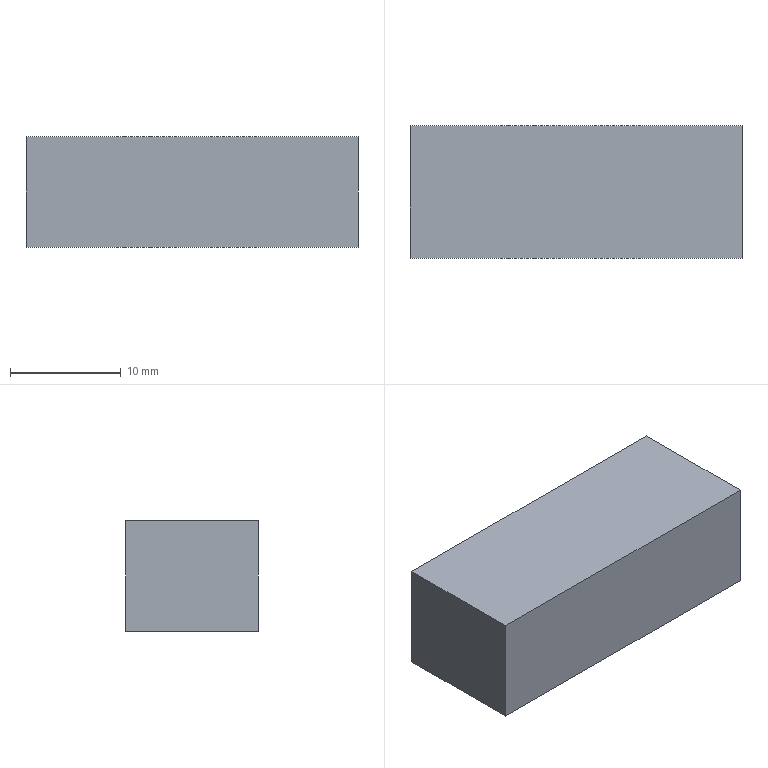Part | SolidWorks | features Extrusion 1 | 1 solid | 6 faces | box 30 x 12 x 10 mm | volume 3600 mm3 | plane 6
STEP:
#1=CARTESIAN_POINT('',(-15.,6.,5.));
#2=VERTEX_POINT('',#1);
#3=CARTESIAN_POINT('',(-15.,-6.,5.));
#4=VERTEX_POINT('',#3);
#5=CARTESIAN_POINT('',(-15.,6.,5.));
#6=DIRECTION('',(0.,-1.,0.));
#7=VECTOR('',#6,1000.);
#8=LINE('',#5,#7);
#9=EDGE_CURVE('',#2,#4,#8,.T.);
#10=ORIENTED_EDGE('',*,*,#9,.F.);
#11=CARTESIAN_POINT('',(-15.,6.,-5.));
#12=VERTEX_POINT('',#11);
#13=CARTESIAN_POINT('',(-15.,6.,-5.));
#14=DIRECTION('',(0.,0.,1.));
#15=VECTOR('',#14,1000.);
#16=LINE('',#13,#15);
#17=EDGE_CURVE('',#12,#2,#16,.T.);
#18=ORIENTED_EDGE('',*,*,#17,.F.);
#19=CARTESIAN_POINT('',(-15.,-6.,-5.));
#20=VERTEX_POINT('',#19);
#21=CARTESIAN_POINT('',(-15.,6.,-5.));
#22=DIRECTION('',(0.,-1.,0.));
#23=VECTOR('',#22,1000.);
#24=LINE('',#21,#23);
#25=EDGE_CURVE('',#12,#20,#24,.T.);
#26=ORIENTED_EDGE('',*,*,#25,.T.);
#27=CARTESIAN_POINT('',(-15.,-6.,-5.));
#28=DIRECTION('',(0.,0.,1.));
#29=VECTOR('',#28,1000.);
#30=LINE('',#27,#29);
#31=EDGE_CURVE('',#20,#4,#30,.T.);
#32=ORIENTED_EDGE('',*,*,#31,.T.);
#33=EDGE_LOOP('',(#10,#18,#26,#32));
#34=FACE_OUTER_BOUND('',#33,.T.);
#35=CARTESIAN_POINT('',(-15.,6.,-5.));
#36=DIRECTION('',(-1.,0.,0.));
#37=DIRECTION('',(0.,0.,1.));
#38=AXIS2_PLACEMENT_3D('',#35,#36,#37);
#39=PLANE('',#38);
#40=ADVANCED_FACE('',(#34),#39,.T.);
#41=CARTESIAN_POINT('',(15.,6.,5.));
#42=VERTEX_POINT('',#41);
#43=CARTESIAN_POINT('',(15.,6.,5.));
#44=DIRECTION('',(-1.,0.,0.));
#45=VECTOR('',#44,1000.);
#46=LINE('',#43,#45);
#47=EDGE_CURVE('',#42,#2,#46,.T.);
#48=ORIENTED_EDGE('',*,*,#47,.F.);
#49=CARTESIAN_POINT('',(15.,6.,-5.));
#50=VERTEX_POINT('',#49);
#51=CARTESIAN_POINT('',(15.,6.,-5.));
#52=DIRECTION('',(0.,0.,1.));
#53=VECTOR('',#52,1000.);
#54=LINE('',#51,#53);
#55=EDGE_CURVE('',#50,#42,#54,.T.);
#56=ORIENTED_EDGE('',*,*,#55,.F.);
#57=CARTESIAN_POINT('',(15.,6.,-5.));
#58=DIRECTION('',(-1.,0.,0.));
#59=VECTOR('',#58,1000.);
#60=LINE('',#57,#59);
#61=EDGE_CURVE('',#50,#12,#60,.T.);
#62=ORIENTED_EDGE('',*,*,#61,.T.);
#63=ORIENTED_EDGE('',*,*,#17,.T.);
#64=EDGE_LOOP('',(#48,#56,#62,#63));
#65=FACE_OUTER_BOUND('',#64,.T.);
#66=CARTESIAN_POINT('',(15.,6.,-5.));
#67=DIRECTION('',(0.,1.,0.));
#68=DIRECTION('',(0.,0.,1.));
#69=AXIS2_PLACEMENT_3D('',#66,#67,#68);
#70=PLANE('',#69);
#71=ADVANCED_FACE('',(#65),#70,.T.);
#72=CARTESIAN_POINT('',(15.,-6.,5.));
#73=VERTEX_POINT('',#72);
#74=CARTESIAN_POINT('',(15.,-6.,5.));
#75=DIRECTION('',(0.,1.,0.));
#76=VECTOR('',#75,1000.);
#77=LINE('',#74,#76);
#78=EDGE_CURVE('',#73,#42,#77,.T.);
#79=ORIENTED_EDGE('',*,*,#78,.F.);
#80=CARTESIAN_POINT('',(15.,-6.,-5.));
#81=VERTEX_POINT('',#80);
#82=CARTESIAN_POINT('',(15.,-6.,-5.));
#83=DIRECTION('',(0.,0.,1.));
#84=VECTOR('',#83,1000.);
#85=LINE('',#82,#84);
#86=EDGE_CURVE('',#81,#73,#85,.T.);
#87=ORIENTED_EDGE('',*,*,#86,.F.);
#88=CARTESIAN_POINT('',(15.,-6.,-5.));
#89=DIRECTION('',(0.,1.,0.));
#90=VECTOR('',#89,1000.);
#91=LINE('',#88,#90);
#92=EDGE_CURVE('',#81,#50,#91,.T.);
#93=ORIENTED_EDGE('',*,*,#92,.T.);
#94=ORIENTED_EDGE('',*,*,#55,.T.);
#95=EDGE_LOOP('',(#79,#87,#93,#94));
#96=FACE_OUTER_BOUND('',#95,.T.);
#97=CARTESIAN_POINT('',(15.,-6.,-5.));
#98=DIRECTION('',(1.,0.,0.));
#99=DIRECTION('',(0.,0.,-1.));
#100=AXIS2_PLACEMENT_3D('',#97,#98,#99);
#101=PLANE('',#100);
#102=ADVANCED_FACE('',(#96),#101,.T.);
#103=CARTESIAN_POINT('',(-15.,-6.,5.));
#104=DIRECTION('',(1.,0.,0.));
#105=VECTOR('',#104,1000.);
#106=LINE('',#103,#105);
#107=EDGE_CURVE('',#4,#73,#106,.T.);
#108=ORIENTED_EDGE('',*,*,#107,.F.);
#109=ORIENTED_EDGE('',*,*,#31,.F.);
#110=CARTESIAN_POINT('',(-15.,-6.,-5.));
#111=DIRECTION('',(1.,0.,0.));
#112=VECTOR('',#111,1000.);
#113=LINE('',#110,#112);
#114=EDGE_CURVE('',#20,#81,#113,.T.);
#115=ORIENTED_EDGE('',*,*,#114,.T.);
#116=ORIENTED_EDGE('',*,*,#86,.T.);
#117=EDGE_LOOP('',(#108,#109,#115,#116));
#118=FACE_OUTER_BOUND('',#117,.T.);
#119=CARTESIAN_POINT('',(-15.,-6.,-5.));
#120=DIRECTION('',(0.,-1.,0.));
#121=DIRECTION('',(0.,0.,-1.));
#122=AXIS2_PLACEMENT_3D('',#119,#120,#121);
#123=PLANE('',#122);
#124=ADVANCED_FACE('',(#118),#123,.T.);
#125=ORIENTED_EDGE('',*,*,#25,.F.);
#126=ORIENTED_EDGE('',*,*,#61,.F.);
#127=ORIENTED_EDGE('',*,*,#92,.F.);
#128=ORIENTED_EDGE('',*,*,#114,.F.);
#129=EDGE_LOOP('',(#125,#126,#127,#128));
#130=FACE_OUTER_BOUND('',#129,.T.);
#131=CARTESIAN_POINT('',(0.,0.,-5.));
#132=DIRECTION('',(0.,0.,1.));
#133=DIRECTION('',(1.,0.,0.));
#134=AXIS2_PLACEMENT_3D('',#131,#132,#133);
#135=PLANE('',#134);
#136=ADVANCED_FACE('',(#130),#135,.F.);
#137=ORIENTED_EDGE('',*,*,#9,.T.);
#138=ORIENTED_EDGE('',*,*,#107,.T.);
#139=ORIENTED_EDGE('',*,*,#78,.T.);
#140=ORIENTED_EDGE('',*,*,#47,.T.);
#141=EDGE_LOOP('',(#137,#138,#139,#140));
#142=FACE_OUTER_BOUND('',#141,.T.);
#143=CARTESIAN_POINT('',(0.,0.,5.));
#144=DIRECTION('',(0.,0.,1.));
#145=DIRECTION('',(1.,0.,0.));
#146=AXIS2_PLACEMENT_3D('',#143,#144,#145);
#147=PLANE('',#146);
#148=ADVANCED_FACE('',(#142),#147,.T.);
#149=CLOSED_SHELL('',(#40,#71,#102,#124,#136,#148));
#150=MANIFOLD_SOLID_BREP('',#149);
#151=CARTESIAN_POINT('',(0.,0.,0.));
#152=DIRECTION('',(0.,0.,1.));
#153=DIRECTION('',(1.,0.,0.));
#154=AXIS2_PLACEMENT_3D('',#151,#152,#153);
#155=(LENGTH_UNIT()NAMED_UNIT(*)SI_UNIT(.MILLI.,.METRE.));
#156=UNCERTAINTY_MEASURE_WITH_UNIT(LENGTH_MEASURE(0.00001),#155,'','');
#157=(NAMED_UNIT(*)PLANE_ANGLE_UNIT()SI_UNIT($,.RADIAN.));
#158=(NAMED_UNIT(*)SI_UNIT($,.STERADIAN.)SOLID_ANGLE_UNIT());
#159=(GEOMETRIC_REPRESENTATION_CONTEXT(3)GLOBAL_UNCERTAINTY_ASSIGNED_CONTEXT((#156))GLOBAL_UNIT_ASSIGNED_CONTEXT((#155,#157,#158))REPRESENTATION_CONTEXT('',''));
#160=ADVANCED_BREP_SHAPE_REPRESENTATION('',(#150,#154),#159);